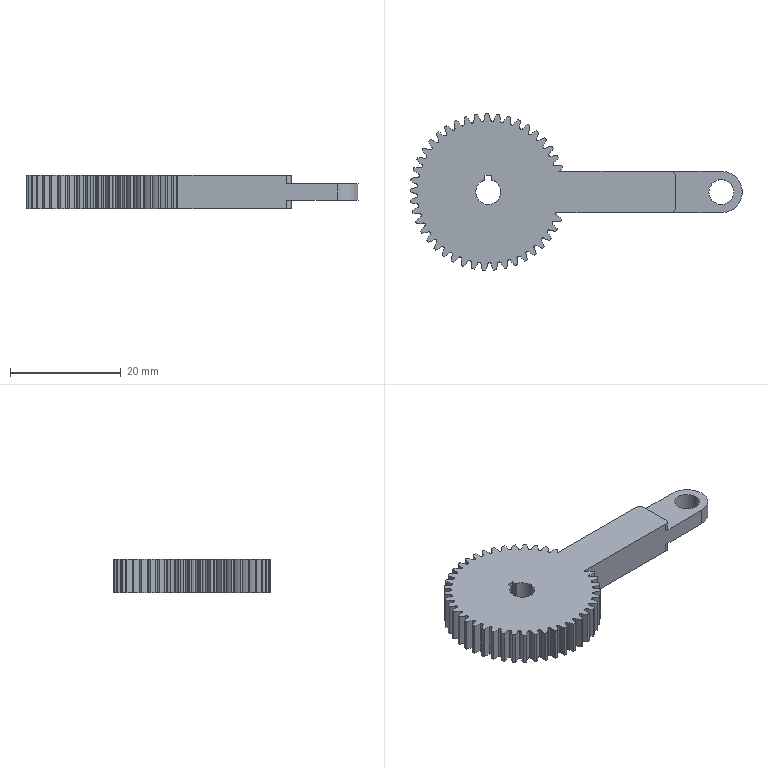Part | SolidWorks | features Extrusion 1, Fillet 1, ICE 1, Scale 1 | 1 solid | 285 faces | box 59.85 x 28.19 x 6 mm | volume 4440 mm3 | cylinder 274 | plane 11 | commonest cylinder face diameters 0.6 x96 8.958 x43 9.083 x42 25.5 x41 28.2 x41 4.5 x5